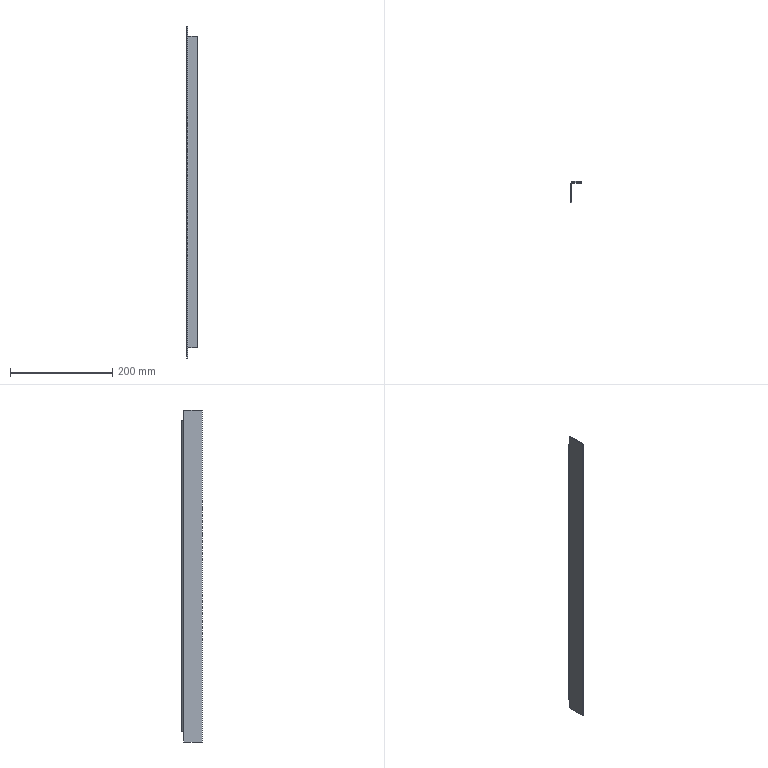Part | SolidWorks | features SMBaseFlange 2, FlatPattern 1, SheetMetal 1 | 1 solid | 16 faces | box 20 x 40 x 649 mm | volume 71956 mm3 | plane 14 | cylinder 2 | commonest cylinder face diameters 4 x1 8 x1
STEP:
#1=CARTESIAN_POINT('',(4.,40.,609.));
#2=VERTEX_POINT('',#1);
#3=CARTESIAN_POINT('',(4.,38.,609.));
#4=VERTEX_POINT('',#3);
#5=CARTESIAN_POINT('',(4.,40.,609.));
#6=DIRECTION('',(0.,-1.,0.));
#7=VECTOR('',#6,1000.);
#8=LINE('',#5,#7);
#9=EDGE_CURVE('',#2,#4,#8,.T.);
#10=ORIENTED_EDGE('',*,*,#9,.F.);
#11=CARTESIAN_POINT('',(0.,36.,609.));
#12=VERTEX_POINT('',#11);
#13=CARTESIAN_POINT('',(4.,36.,609.));
#14=DIRECTION('',(0.,0.,-1.));
#15=DIRECTION('',(1.,0.,0.));
#16=AXIS2_PLACEMENT_3D('',#13,#14,#15);
#17=CIRCLE('',#16,4.);
#18=EDGE_CURVE('',#12,#2,#17,.T.);
#19=ORIENTED_EDGE('',*,*,#18,.F.);
#20=CARTESIAN_POINT('',(2.,36.,609.));
#21=VERTEX_POINT('',#20);
#22=CARTESIAN_POINT('',(2.,36.,609.));
#23=DIRECTION('',(-1.,0.,0.));
#24=VECTOR('',#23,1000.);
#25=LINE('',#22,#24);
#26=EDGE_CURVE('',#21,#12,#25,.T.);
#27=ORIENTED_EDGE('',*,*,#26,.F.);
#28=CARTESIAN_POINT('',(4.,36.,609.));
#29=DIRECTION('',(0.,0.,-1.));
#30=DIRECTION('',(1.,0.,0.));
#31=AXIS2_PLACEMENT_3D('',#28,#29,#30);
#32=CIRCLE('',#31,2.);
#33=EDGE_CURVE('',#21,#4,#32,.T.);
#34=ORIENTED_EDGE('',*,*,#33,.T.);
#35=EDGE_LOOP('',(#10,#19,#27,#34));
#36=FACE_OUTER_BOUND('',#35,.T.);
#37=CARTESIAN_POINT('',(4.,40.,609.));
#38=DIRECTION('',(0.,0.,1.));
#39=DIRECTION('',(1.,0.,0.));
#40=AXIS2_PLACEMENT_3D('',#37,#38,#39);
#41=PLANE('',#40);
#42=ADVANCED_FACE('',(#36),#41,.T.);
#43=CARTESIAN_POINT('',(20.,40.,609.));
#44=VERTEX_POINT('',#43);
#45=CARTESIAN_POINT('',(0.,40.,609.));
#46=DIRECTION('',(1.,0.,0.));
#47=VECTOR('',#46,1000.);
#48=LINE('',#45,#47);
#49=EDGE_CURVE('',#2,#44,#48,.T.);
#50=ORIENTED_EDGE('',*,*,#49,.F.);
#51=ORIENTED_EDGE('',*,*,#9,.T.);
#52=CARTESIAN_POINT('',(20.,38.,609.));
#53=VERTEX_POINT('',#52);
#54=CARTESIAN_POINT('',(0.,38.,609.));
#55=DIRECTION('',(1.,0.,0.));
#56=VECTOR('',#55,1000.);
#57=LINE('',#54,#56);
#58=EDGE_CURVE('',#4,#53,#57,.T.);
#59=ORIENTED_EDGE('',*,*,#58,.T.);
#60=CARTESIAN_POINT('',(20.,40.,609.));
#61=DIRECTION('',(0.,-1.,0.));
#62=VECTOR('',#61,1000.);
#63=LINE('',#60,#62);
#64=EDGE_CURVE('',#44,#53,#63,.T.);
#65=ORIENTED_EDGE('',*,*,#64,.F.);
#66=EDGE_LOOP('',(#50,#51,#59,#65));
#67=FACE_OUTER_BOUND('',#66,.T.);
#68=CARTESIAN_POINT('',(2.,36.,609.));
#69=DIRECTION('',(0.,0.,1.));
#70=DIRECTION('',(1.,0.,0.));
#71=AXIS2_PLACEMENT_3D('',#68,#69,#70);
#72=PLANE('',#71);
#73=ADVANCED_FACE('',(#67),#72,.T.);
#74=CARTESIAN_POINT('',(0.,36.,0.));
#75=VERTEX_POINT('',#74);
#76=CARTESIAN_POINT('',(2.,36.,0.));
#77=VERTEX_POINT('',#76);
#78=CARTESIAN_POINT('',(0.,36.,0.));
#79=DIRECTION('',(1.,0.,0.));
#80=VECTOR('',#79,1000.);
#81=LINE('',#78,#80);
#82=EDGE_CURVE('',#75,#77,#81,.T.);
#83=ORIENTED_EDGE('',*,*,#82,.F.);
#84=CARTESIAN_POINT('',(4.,40.,0.));
#85=VERTEX_POINT('',#84);
#86=CARTESIAN_POINT('',(4.,36.,0.));
#87=DIRECTION('',(0.,0.,-1.));
#88=DIRECTION('',(1.,0.,0.));
#89=AXIS2_PLACEMENT_3D('',#86,#87,#88);
#90=CIRCLE('',#89,4.);
#91=EDGE_CURVE('',#75,#85,#90,.T.);
#92=ORIENTED_EDGE('',*,*,#91,.T.);
#93=CARTESIAN_POINT('',(4.,38.,0.));
#94=VERTEX_POINT('',#93);
#95=CARTESIAN_POINT('',(4.,38.,0.));
#96=DIRECTION('',(0.,1.,0.));
#97=VECTOR('',#96,1000.);
#98=LINE('',#95,#97);
#99=EDGE_CURVE('',#94,#85,#98,.T.);
#100=ORIENTED_EDGE('',*,*,#99,.F.);
#101=CARTESIAN_POINT('',(4.,36.,0.));
#102=DIRECTION('',(0.,0.,-1.));
#103=DIRECTION('',(1.,0.,0.));
#104=AXIS2_PLACEMENT_3D('',#101,#102,#103);
#105=CIRCLE('',#104,2.);
#106=EDGE_CURVE('',#77,#94,#105,.T.);
#107=ORIENTED_EDGE('',*,*,#106,.F.);
#108=EDGE_LOOP('',(#83,#92,#100,#107));
#109=FACE_OUTER_BOUND('',#108,.T.);
#110=CARTESIAN_POINT('',(0.,36.,0.));
#111=DIRECTION('',(0.,0.,-1.));
#112=DIRECTION('',(-1.,0.,0.));
#113=AXIS2_PLACEMENT_3D('',#110,#111,#112);
#114=PLANE('',#113);
#115=ADVANCED_FACE('',(#109),#114,.T.);
#116=CARTESIAN_POINT('',(20.,38.,0.));
#117=VERTEX_POINT('',#116);
#118=CARTESIAN_POINT('',(0.,38.,0.));
#119=DIRECTION('',(1.,0.,0.));
#120=VECTOR('',#119,1000.);
#121=LINE('',#118,#120);
#122=EDGE_CURVE('',#94,#117,#121,.T.);
#123=ORIENTED_EDGE('',*,*,#122,.T.);
#124=CARTESIAN_POINT('',(20.,38.,609.));
#125=DIRECTION('',(0.,0.,-1.));
#126=VECTOR('',#125,1000.);
#127=LINE('',#124,#126);
#128=EDGE_CURVE('',#53,#117,#127,.T.);
#129=ORIENTED_EDGE('',*,*,#128,.F.);
#130=ORIENTED_EDGE('',*,*,#58,.F.);
#131=CARTESIAN_POINT('',(4.,38.,609.));
#132=DIRECTION('',(0.,0.,-1.));
#133=VECTOR('',#132,1000.);
#134=LINE('',#131,#133);
#135=EDGE_CURVE('',#4,#94,#134,.T.);
#136=ORIENTED_EDGE('',*,*,#135,.T.);
#137=EDGE_LOOP('',(#123,#129,#130,#136));
#138=FACE_OUTER_BOUND('',#137,.T.);
#139=CARTESIAN_POINT('',(0.,38.,609.));
#140=DIRECTION('',(0.,1.,0.));
#141=DIRECTION('',(0.,0.,1.));
#142=AXIS2_PLACEMENT_3D('',#139,#140,#141);
#143=PLANE('',#142);
#144=ADVANCED_FACE('',(#138),#143,.F.);
#145=CARTESIAN_POINT('',(20.,40.,0.));
#146=VERTEX_POINT('',#145);
#147=CARTESIAN_POINT('',(20.,40.,0.));
#148=DIRECTION('',(0.,-1.,0.));
#149=VECTOR('',#148,1000.);
#150=LINE('',#147,#149);
#151=EDGE_CURVE('',#146,#117,#150,.T.);
#152=ORIENTED_EDGE('',*,*,#151,.F.);
#153=CARTESIAN_POINT('',(20.,40.,609.));
#154=DIRECTION('',(0.,0.,-1.));
#155=VECTOR('',#154,1000.);
#156=LINE('',#153,#155);
#157=EDGE_CURVE('',#44,#146,#156,.T.);
#158=ORIENTED_EDGE('',*,*,#157,.F.);
#159=ORIENTED_EDGE('',*,*,#64,.T.);
#160=ORIENTED_EDGE('',*,*,#128,.T.);
#161=EDGE_LOOP('',(#152,#158,#159,#160));
#162=FACE_OUTER_BOUND('',#161,.T.);
#163=CARTESIAN_POINT('',(20.,40.,609.));
#164=DIRECTION('',(1.,0.,0.));
#165=DIRECTION('',(0.,0.,-1.));
#166=AXIS2_PLACEMENT_3D('',#163,#164,#165);
#167=PLANE('',#166);
#168=ADVANCED_FACE('',(#162),#167,.T.);
#169=CARTESIAN_POINT('',(0.,40.,0.));
#170=DIRECTION('',(1.,0.,0.));
#171=VECTOR('',#170,1000.);
#172=LINE('',#169,#171);
#173=EDGE_CURVE('',#85,#146,#172,.T.);
#174=ORIENTED_EDGE('',*,*,#173,.F.);
#175=CARTESIAN_POINT('',(4.,40.,609.));
#176=DIRECTION('',(0.,0.,-1.));
#177=VECTOR('',#176,1000.);
#178=LINE('',#175,#177);
#179=EDGE_CURVE('',#2,#85,#178,.T.);
#180=ORIENTED_EDGE('',*,*,#179,.F.);
#181=ORIENTED_EDGE('',*,*,#49,.T.);
#182=ORIENTED_EDGE('',*,*,#157,.T.);
#183=EDGE_LOOP('',(#174,#180,#181,#182));
#184=FACE_OUTER_BOUND('',#183,.T.);
#185=CARTESIAN_POINT('',(0.,40.,609.));
#186=DIRECTION('',(0.,1.,0.));
#187=DIRECTION('',(0.,0.,1.));
#188=AXIS2_PLACEMENT_3D('',#185,#186,#187);
#189=PLANE('',#188);
#190=ADVANCED_FACE('',(#184),#189,.T.);
#191=ORIENTED_EDGE('',*,*,#91,.F.);
#192=CARTESIAN_POINT('',(0.,36.,609.));
#193=DIRECTION('',(0.,0.,-1.));
#194=VECTOR('',#193,1000.);
#195=LINE('',#192,#194);
#196=EDGE_CURVE('',#12,#75,#195,.T.);
#197=ORIENTED_EDGE('',*,*,#196,.F.);
#198=ORIENTED_EDGE('',*,*,#18,.T.);
#199=ORIENTED_EDGE('',*,*,#179,.T.);
#200=EDGE_LOOP('',(#191,#197,#198,#199));
#201=FACE_OUTER_BOUND('',#200,.T.);
#202=CARTESIAN_POINT('',(4.,36.,609.));
#203=DIRECTION('',(0.,0.,-1.));
#204=DIRECTION('',(-1.,0.,0.));
#205=AXIS2_PLACEMENT_3D('',#202,#203,#204);
#206=CYLINDRICAL_SURFACE('',#205,4.);
#207=ADVANCED_FACE('',(#201),#206,.T.);
#208=ORIENTED_EDGE('',*,*,#196,.T.);
#209=CARTESIAN_POINT('',(0.,36.,-20.));
#210=VERTEX_POINT('',#209);
#211=CARTESIAN_POINT('',(0.,36.,0.));
#212=DIRECTION('',(0.,0.,1.));
#213=VECTOR('',#212,1000.);
#214=LINE('',#211,#213);
#215=EDGE_CURVE('',#210,#75,#214,.T.);
#216=ORIENTED_EDGE('',*,*,#215,.F.);
#217=CARTESIAN_POINT('',(0.,0.,-20.));
#218=VERTEX_POINT('',#217);
#219=CARTESIAN_POINT('',(0.,0.,-20.));
#220=DIRECTION('',(0.,1.,0.));
#221=VECTOR('',#220,1000.);
#222=LINE('',#219,#221);
#223=EDGE_CURVE('',#218,#210,#222,.T.);
#224=ORIENTED_EDGE('',*,*,#223,.F.);
#225=CARTESIAN_POINT('',(0.,0.,629.));
#226=VERTEX_POINT('',#225);
#227=CARTESIAN_POINT('',(0.,0.,609.));
#228=DIRECTION('',(0.,0.,-1.));
#229=VECTOR('',#228,1000.);
#230=LINE('',#227,#229);
#231=EDGE_CURVE('',#226,#218,#230,.T.);
#232=ORIENTED_EDGE('',*,*,#231,.F.);
#233=CARTESIAN_POINT('',(0.,36.,629.));
#234=VERTEX_POINT('',#233);
#235=CARTESIAN_POINT('',(0.,0.,629.));
#236=DIRECTION('',(0.,-1.,0.));
#237=VECTOR('',#236,1000.);
#238=LINE('',#235,#237);
#239=EDGE_CURVE('',#234,#226,#238,.T.);
#240=ORIENTED_EDGE('',*,*,#239,.F.);
#241=CARTESIAN_POINT('',(0.,36.,609.));
#242=DIRECTION('',(0.,0.,1.));
#243=VECTOR('',#242,1000.);
#244=LINE('',#241,#243);
#245=EDGE_CURVE('',#12,#234,#244,.T.);
#246=ORIENTED_EDGE('',*,*,#245,.F.);
#247=EDGE_LOOP('',(#208,#216,#224,#232,#240,#246));
#248=FACE_OUTER_BOUND('',#247,.T.);
#249=CARTESIAN_POINT('',(0.,0.,609.));
#250=DIRECTION('',(-1.,0.,0.));
#251=DIRECTION('',(0.,0.,1.));
#252=AXIS2_PLACEMENT_3D('',#249,#250,#251);
#253=PLANE('',#252);
#254=ADVANCED_FACE('',(#248),#253,.T.);
#255=ORIENTED_EDGE('',*,*,#231,.T.);
#256=CARTESIAN_POINT('',(2.,0.,-20.));
#257=VERTEX_POINT('',#256);
#258=CARTESIAN_POINT('',(0.,0.,-20.));
#259=DIRECTION('',(1.,0.,0.));
#260=VECTOR('',#259,1000.);
#261=LINE('',#258,#260);
#262=EDGE_CURVE('',#218,#257,#261,.T.);
#263=ORIENTED_EDGE('',*,*,#262,.T.);
#264=CARTESIAN_POINT('',(2.,0.,629.));
#265=VERTEX_POINT('',#264);
#266=CARTESIAN_POINT('',(2.,0.,609.));
#267=DIRECTION('',(0.,0.,-1.));
#268=VECTOR('',#267,1000.);
#269=LINE('',#266,#268);
#270=EDGE_CURVE('',#265,#257,#269,.T.);
#271=ORIENTED_EDGE('',*,*,#270,.F.);
#272=CARTESIAN_POINT('',(0.,0.,629.));
#273=DIRECTION('',(1.,0.,0.));
#274=VECTOR('',#273,1000.);
#275=LINE('',#272,#274);
#276=EDGE_CURVE('',#226,#265,#275,.T.);
#277=ORIENTED_EDGE('',*,*,#276,.F.);
#278=EDGE_LOOP('',(#255,#263,#271,#277));
#279=FACE_OUTER_BOUND('',#278,.T.);
#280=CARTESIAN_POINT('',(2.,0.,609.));
#281=DIRECTION('',(0.,-1.,0.));
#282=DIRECTION('',(0.,0.,-1.));
#283=AXIS2_PLACEMENT_3D('',#280,#281,#282);
#284=PLANE('',#283);
#285=ADVANCED_FACE('',(#279),#284,.T.);
#286=ORIENTED_EDGE('',*,*,#270,.T.);
#287=CARTESIAN_POINT('',(2.,36.,-20.));
#288=VERTEX_POINT('',#287);
#289=CARTESIAN_POINT('',(2.,0.,-20.));
#290=DIRECTION('',(0.,1.,0.));
#291=VECTOR('',#290,1000.);
#292=LINE('',#289,#291);
#293=EDGE_CURVE('',#257,#288,#292,.T.);
#294=ORIENTED_EDGE('',*,*,#293,.T.);
#295=CARTESIAN_POINT('',(2.,36.,0.));
#296=DIRECTION('',(0.,0.,1.));
#297=VECTOR('',#296,1000.);
#298=LINE('',#295,#297);
#299=EDGE_CURVE('',#288,#77,#298,.T.);
#300=ORIENTED_EDGE('',*,*,#299,.T.);
#301=CARTESIAN_POINT('',(2.,36.,609.));
#302=DIRECTION('',(0.,0.,-1.));
#303=VECTOR('',#302,1000.);
#304=LINE('',#301,#303);
#305=EDGE_CURVE('',#21,#77,#304,.T.);
#306=ORIENTED_EDGE('',*,*,#305,.F.);
#307=CARTESIAN_POINT('',(2.,36.,629.));
#308=VERTEX_POINT('',#307);
#309=CARTESIAN_POINT('',(2.,36.,609.));
#310=DIRECTION('',(0.,0.,1.));
#311=VECTOR('',#310,1000.);
#312=LINE('',#309,#311);
#313=EDGE_CURVE('',#21,#308,#312,.T.);
#314=ORIENTED_EDGE('',*,*,#313,.T.);
#315=CARTESIAN_POINT('',(2.,0.,629.));
#316=DIRECTION('',(0.,-1.,0.));
#317=VECTOR('',#316,1000.);
#318=LINE('',#315,#317);
#319=EDGE_CURVE('',#308,#265,#318,.T.);
#320=ORIENTED_EDGE('',*,*,#319,.T.);
#321=EDGE_LOOP('',(#286,#294,#300,#306,#314,#320));
#322=FACE_OUTER_BOUND('',#321,.T.);
#323=CARTESIAN_POINT('',(2.,0.,609.));
#324=DIRECTION('',(-1.,0.,0.));
#325=DIRECTION('',(0.,0.,1.));
#326=AXIS2_PLACEMENT_3D('',#323,#324,#325);
#327=PLANE('',#326);
#328=ADVANCED_FACE('',(#322),#327,.F.);
#329=ORIENTED_EDGE('',*,*,#106,.T.);
#330=ORIENTED_EDGE('',*,*,#135,.F.);
#331=ORIENTED_EDGE('',*,*,#33,.F.);
#332=ORIENTED_EDGE('',*,*,#305,.T.);
#333=EDGE_LOOP('',(#329,#330,#331,#332));
#334=FACE_OUTER_BOUND('',#333,.T.);
#335=CARTESIAN_POINT('',(4.,36.,609.));
#336=DIRECTION('',(0.,0.,-1.));
#337=DIRECTION('',(-1.,0.,0.));
#338=AXIS2_PLACEMENT_3D('',#335,#336,#337);
#339=CYLINDRICAL_SURFACE('',#338,2.);
#340=ADVANCED_FACE('',(#334),#339,.F.);
#341=ORIENTED_EDGE('',*,*,#122,.F.);
#342=ORIENTED_EDGE('',*,*,#99,.T.);
#343=ORIENTED_EDGE('',*,*,#173,.T.);
#344=ORIENTED_EDGE('',*,*,#151,.T.);
#345=EDGE_LOOP('',(#341,#342,#343,#344));
#346=FACE_OUTER_BOUND('',#345,.T.);
#347=CARTESIAN_POINT('',(4.,36.,0.));
#348=DIRECTION('',(0.,0.,1.));
#349=DIRECTION('',(1.,0.,0.));
#350=AXIS2_PLACEMENT_3D('',#347,#348,#349);
#351=PLANE('',#350);
#352=ADVANCED_FACE('',(#346),#351,.F.);
#353=ORIENTED_EDGE('',*,*,#319,.F.);
#354=CARTESIAN_POINT('',(0.,36.,629.));
#355=DIRECTION('',(1.,0.,0.));
#356=VECTOR('',#355,1000.);
#357=LINE('',#354,#356);
#358=EDGE_CURVE('',#234,#308,#357,.T.);
#359=ORIENTED_EDGE('',*,*,#358,.F.);
#360=ORIENTED_EDGE('',*,*,#239,.T.);
#361=ORIENTED_EDGE('',*,*,#276,.T.);
#362=EDGE_LOOP('',(#353,#359,#360,#361));
#363=FACE_OUTER_BOUND('',#362,.T.);
#364=CARTESIAN_POINT('',(0.,0.,629.));
#365=DIRECTION('',(0.,0.,1.));
#366=DIRECTION('',(1.,0.,0.));
#367=AXIS2_PLACEMENT_3D('',#364,#365,#366);
#368=PLANE('',#367);
#369=ADVANCED_FACE('',(#363),#368,.T.);
#370=ORIENTED_EDGE('',*,*,#313,.F.);
#371=ORIENTED_EDGE('',*,*,#26,.T.);
#372=ORIENTED_EDGE('',*,*,#245,.T.);
#373=ORIENTED_EDGE('',*,*,#358,.T.);
#374=EDGE_LOOP('',(#370,#371,#372,#373));
#375=FACE_OUTER_BOUND('',#374,.T.);
#376=CARTESIAN_POINT('',(0.,36.,609.));
#377=DIRECTION('',(0.,1.,0.));
#378=DIRECTION('',(0.,0.,1.));
#379=AXIS2_PLACEMENT_3D('',#376,#377,#378);
#380=PLANE('',#379);
#381=ADVANCED_FACE('',(#375),#380,.T.);
#382=ORIENTED_EDGE('',*,*,#299,.F.);
#383=CARTESIAN_POINT('',(0.,36.,-20.));
#384=DIRECTION('',(1.,0.,0.));
#385=VECTOR('',#384,1000.);
#386=LINE('',#383,#385);
#387=EDGE_CURVE('',#210,#288,#386,.T.);
#388=ORIENTED_EDGE('',*,*,#387,.F.);
#389=ORIENTED_EDGE('',*,*,#215,.T.);
#390=ORIENTED_EDGE('',*,*,#82,.T.);
#391=EDGE_LOOP('',(#382,#388,#389,#390));
#392=FACE_OUTER_BOUND('',#391,.T.);
#393=CARTESIAN_POINT('',(0.,36.,0.));
#394=DIRECTION('',(0.,1.,0.));
#395=DIRECTION('',(0.,0.,1.));
#396=AXIS2_PLACEMENT_3D('',#393,#394,#395);
#397=PLANE('',#396);
#398=ADVANCED_FACE('',(#392),#397,.T.);
#399=ORIENTED_EDGE('',*,*,#293,.F.);
#400=ORIENTED_EDGE('',*,*,#262,.F.);
#401=ORIENTED_EDGE('',*,*,#223,.T.);
#402=ORIENTED_EDGE('',*,*,#387,.T.);
#403=EDGE_LOOP('',(#399,#400,#401,#402));
#404=FACE_OUTER_BOUND('',#403,.T.);
#405=CARTESIAN_POINT('',(0.,0.,-20.));
#406=DIRECTION('',(0.,0.,-1.));
#407=DIRECTION('',(-1.,0.,0.));
#408=AXIS2_PLACEMENT_3D('',#405,#406,#407);
#409=PLANE('',#408);
#410=ADVANCED_FACE('',(#404),#409,.T.);
#411=CLOSED_SHELL('',(#42,#73,#115,#144,#168,#190,#207,#254,#285,#328,#340,#352,#369,#381,#398,#410));
#412=MANIFOLD_SOLID_BREP('',#411);
#413=CARTESIAN_POINT('',(0.,0.,0.));
#414=DIRECTION('',(0.,0.,1.));
#415=DIRECTION('',(1.,0.,0.));
#416=AXIS2_PLACEMENT_3D('',#413,#414,#415);
#417=(LENGTH_UNIT()NAMED_UNIT(*)SI_UNIT(.MILLI.,.METRE.));
#418=UNCERTAINTY_MEASURE_WITH_UNIT(LENGTH_MEASURE(0.00001),#417,'','');
#419=(NAMED_UNIT(*)PLANE_ANGLE_UNIT()SI_UNIT($,.RADIAN.));
#420=(NAMED_UNIT(*)SI_UNIT($,.STERADIAN.)SOLID_ANGLE_UNIT());
#421=(GEOMETRIC_REPRESENTATION_CONTEXT(3)GLOBAL_UNCERTAINTY_ASSIGNED_CONTEXT((#418))GLOBAL_UNIT_ASSIGNED_CONTEXT((#417,#419,#420))REPRESENTATION_CONTEXT('',''));
#422=ADVANCED_BREP_SHAPE_REPRESENTATION('',(#412,#416),#421);